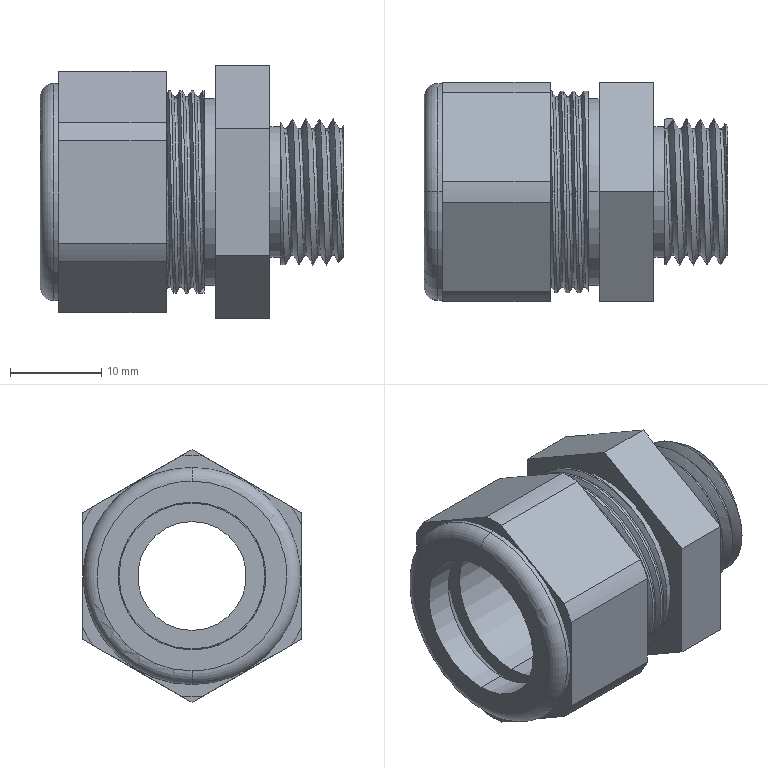Part | SolidWorks | features BaseBody 1 | 1 solid | 92 faces | box 33.25 x 24 x 27.713 mm | volume 7820 mm3 | cylinder 44 | plane 26 | cone 12 | spline 8 | torus 2 | commonest cylinder face diameters 21 x13 22.2 x8 26.5 x7 16 x4 20.5 x4 11.92 x2